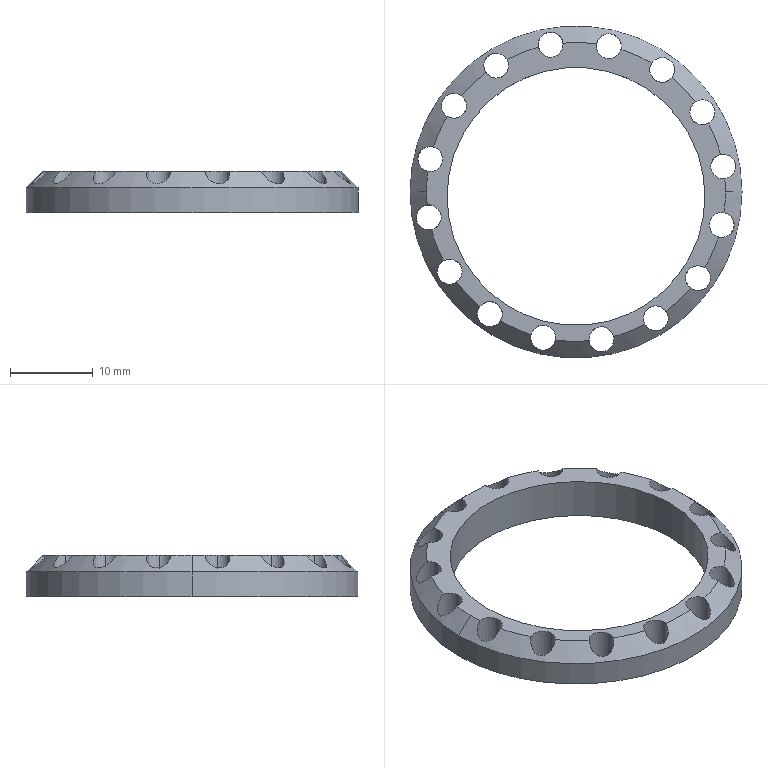Part | SolidWorks | features Chamfer 1, Cut 1, Extrusion 1 | 1 solid | 40 faces | box 40 x 40 x 5 mm | volume 1718 mm3 | cylinder 36 | cone 2 | plane 2 | commonest cylinder face diameters 3 x32 31.082 x2 40 x2